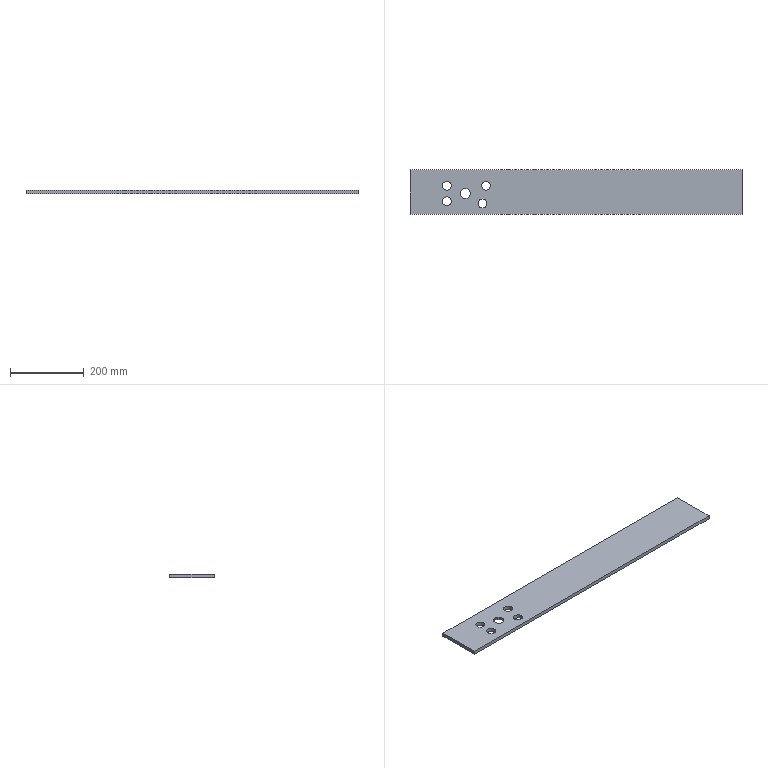Part | STEP file | zhiheceban1 | 1 solid | 13 faces | box 900 x 120 x 10 mm | volume 1052932 mm3 | plane 7 | cylinder 6 | commonest cylinder face diameters 24 x4 28 x1 36 x1
STEP:
#1=CARTESIAN_POINT('',(0.,0.,0.));
#2=DIRECTION('',(0.,0.,1.));
#3=DIRECTION('',(1.,0.,0.));
#4=AXIS2_PLACEMENT_3D('',#1,#2,#3);
#5=CARTESIAN_POINT('',(450.,-60.,-5.));
#6=VERTEX_POINT('',#5);
#7=CARTESIAN_POINT('',(450.,60.,-5.));
#8=VERTEX_POINT('',#7);
#9=CARTESIAN_POINT('',(450.,60.,-5.));
#10=DIRECTION('',(0.,1.,0.));
#11=VECTOR('',#10,1.);
#12=LINE('',#9,#11);
#13=CARTESIAN_POINT('',(450.,60.,5.));
#14=DIRECTION('',(-1.,0.,0.));
#15=DIRECTION('',(0.,0.,1.));
#16=AXIS2_PLACEMENT_3D('',#13,#14,#15);
#17=PLANE('',#16);
#18=CARTESIAN_POINT('',(-10.,0.));
#19=DIRECTION('',(0.,1.));
#20=VECTOR('',#19,1.);
#21=LINE('',#18,#20);
#22=(GEOMETRIC_REPRESENTATION_CONTEXT(2)PARAMETRIC_REPRESENTATION_CONTEXT()REPRESENTATION_CONTEXT('',''));
#23=DEFINITIONAL_REPRESENTATION('',(#21),#22);
#24=PCURVE('',#17,#23);
#25=CARTESIAN_POINT('',(0.,0.,-5.));
#26=DIRECTION('',(0.,0.,1.));
#27=DIRECTION('',(1.,0.,0.));
#28=AXIS2_PLACEMENT_3D('',#25,#26,#27);
#29=PLANE('',#28);
#30=CARTESIAN_POINT('',(450.,60.));
#31=DIRECTION('',(0.,1.));
#32=VECTOR('',#31,1.);
#33=LINE('',#30,#32);
#34=(GEOMETRIC_REPRESENTATION_CONTEXT(2)PARAMETRIC_REPRESENTATION_CONTEXT()REPRESENTATION_CONTEXT('',''));
#35=DEFINITIONAL_REPRESENTATION('',(#33),#34);
#36=PCURVE('',#29,#35);
#37=SURFACE_CURVE('',#12,(#24,#36),.PCURVE_S1.);
#38=EDGE_CURVE('',#6,#8,#37,.T.);
#39=ORIENTED_EDGE('',*,*,#38,.T.);
#40=CARTESIAN_POINT('',(450.,60.,5.));
#41=VERTEX_POINT('',#40);
#42=CARTESIAN_POINT('',(450.,60.,5.));
#43=DIRECTION('',(0.,0.,-1.));
#44=VECTOR('',#43,1.);
#45=LINE('',#42,#44);
#46=CARTESIAN_POINT('',(0.,0.));
#47=DIRECTION('',(-1.,0.));
#48=VECTOR('',#47,1.);
#49=LINE('',#46,#48);
#50=(GEOMETRIC_REPRESENTATION_CONTEXT(2)PARAMETRIC_REPRESENTATION_CONTEXT()REPRESENTATION_CONTEXT('',''));
#51=DEFINITIONAL_REPRESENTATION('',(#49),#50);
#52=PCURVE('',#17,#51);
#53=CARTESIAN_POINT('',(-450.,60.,5.));
#54=DIRECTION('',(0.,-1.,0.));
#55=DIRECTION('',(0.,0.,-1.));
#56=AXIS2_PLACEMENT_3D('',#53,#54,#55);
#57=PLANE('',#56);
#58=CARTESIAN_POINT('',(0.,900.));
#59=DIRECTION('',(1.,0.));
#60=VECTOR('',#59,1.);
#61=LINE('',#58,#60);
#62=(GEOMETRIC_REPRESENTATION_CONTEXT(2)PARAMETRIC_REPRESENTATION_CONTEXT()REPRESENTATION_CONTEXT('',''));
#63=DEFINITIONAL_REPRESENTATION('',(#61),#62);
#64=PCURVE('',#57,#63);
#65=SURFACE_CURVE('',#45,(#52,#64),.PCURVE_S1.);
#66=EDGE_CURVE('',#41,#8,#65,.T.);
#67=ORIENTED_EDGE('',*,*,#66,.F.);
#68=CARTESIAN_POINT('',(450.,-60.,5.));
#69=VERTEX_POINT('',#68);
#70=CARTESIAN_POINT('',(450.,60.,5.));
#71=DIRECTION('',(0.,1.,0.));
#72=VECTOR('',#71,1.);
#73=LINE('',#70,#72);
#74=CARTESIAN_POINT('',(0.,0.));
#75=DIRECTION('',(0.,1.));
#76=VECTOR('',#75,1.);
#77=LINE('',#74,#76);
#78=(GEOMETRIC_REPRESENTATION_CONTEXT(2)PARAMETRIC_REPRESENTATION_CONTEXT()REPRESENTATION_CONTEXT('',''));
#79=DEFINITIONAL_REPRESENTATION('',(#77),#78);
#80=PCURVE('',#17,#79);
#81=CARTESIAN_POINT('',(0.,0.,5.));
#82=DIRECTION('',(0.,0.,1.));
#83=DIRECTION('',(1.,0.,0.));
#84=AXIS2_PLACEMENT_3D('',#81,#82,#83);
#85=PLANE('',#84);
#86=CARTESIAN_POINT('',(450.,60.));
#87=DIRECTION('',(0.,1.));
#88=VECTOR('',#87,1.);
#89=LINE('',#86,#88);
#90=(GEOMETRIC_REPRESENTATION_CONTEXT(2)PARAMETRIC_REPRESENTATION_CONTEXT()REPRESENTATION_CONTEXT('',''));
#91=DEFINITIONAL_REPRESENTATION('',(#89),#90);
#92=PCURVE('',#85,#91);
#93=SURFACE_CURVE('',#73,(#80,#92),.PCURVE_S1.);
#94=EDGE_CURVE('',#69,#41,#93,.T.);
#95=ORIENTED_EDGE('',*,*,#94,.F.);
#96=CARTESIAN_POINT('',(450.,-60.,5.));
#97=DIRECTION('',(0.,0.,-1.));
#98=VECTOR('',#97,1.);
#99=LINE('',#96,#98);
#100=CARTESIAN_POINT('',(0.,-120.));
#101=DIRECTION('',(-1.,0.));
#102=VECTOR('',#101,1.);
#103=LINE('',#100,#102);
#104=(GEOMETRIC_REPRESENTATION_CONTEXT(2)PARAMETRIC_REPRESENTATION_CONTEXT()REPRESENTATION_CONTEXT('',''));
#105=DEFINITIONAL_REPRESENTATION('',(#103),#104);
#106=PCURVE('',#17,#105);
#107=CARTESIAN_POINT('',(-450.,-60.,5.));
#108=DIRECTION('',(0.,1.,0.));
#109=DIRECTION('',(0.,0.,1.));
#110=AXIS2_PLACEMENT_3D('',#107,#108,#109);
#111=PLANE('',#110);
#112=CARTESIAN_POINT('',(0.,900.));
#113=DIRECTION('',(-1.,0.));
#114=VECTOR('',#113,1.);
#115=LINE('',#112,#114);
#116=(GEOMETRIC_REPRESENTATION_CONTEXT(2)PARAMETRIC_REPRESENTATION_CONTEXT()REPRESENTATION_CONTEXT('',''));
#117=DEFINITIONAL_REPRESENTATION('',(#115),#116);
#118=PCURVE('',#111,#117);
#119=SURFACE_CURVE('',#99,(#106,#118),.PCURVE_S1.);
#120=EDGE_CURVE('',#69,#6,#119,.T.);
#121=ORIENTED_EDGE('',*,*,#120,.T.);
#122=EDGE_LOOP('',(#39,#67,#95,#121));
#123=FACE_BOUND('',#122,.T.);
#124=ADVANCED_FACE('',(#123),#17,.F.);
#125=CARTESIAN_POINT('',(-450.,60.,-5.));
#126=VERTEX_POINT('',#125);
#127=CARTESIAN_POINT('',(-450.,60.,-5.));
#128=DIRECTION('',(-1.,0.,0.));
#129=VECTOR('',#128,1.);
#130=LINE('',#127,#129);
#131=CARTESIAN_POINT('',(10.,0.));
#132=DIRECTION('',(0.,-1.));
#133=VECTOR('',#132,1.);
#134=LINE('',#131,#133);
#135=(GEOMETRIC_REPRESENTATION_CONTEXT(2)PARAMETRIC_REPRESENTATION_CONTEXT()REPRESENTATION_CONTEXT('',''));
#136=DEFINITIONAL_REPRESENTATION('',(#134),#135);
#137=PCURVE('',#57,#136);
#138=CARTESIAN_POINT('',(-450.,60.));
#139=DIRECTION('',(-1.,0.));
#140=VECTOR('',#139,1.);
#141=LINE('',#138,#140);
#142=(GEOMETRIC_REPRESENTATION_CONTEXT(2)PARAMETRIC_REPRESENTATION_CONTEXT()REPRESENTATION_CONTEXT('',''));
#143=DEFINITIONAL_REPRESENTATION('',(#141),#142);
#144=PCURVE('',#29,#143);
#145=SURFACE_CURVE('',#130,(#137,#144),.PCURVE_S1.);
#146=EDGE_CURVE('',#8,#126,#145,.T.);
#147=ORIENTED_EDGE('',*,*,#146,.T.);
#148=CARTESIAN_POINT('',(-450.,60.,5.));
#149=VERTEX_POINT('',#148);
#150=CARTESIAN_POINT('',(-450.,60.,5.));
#151=DIRECTION('',(0.,0.,-1.));
#152=VECTOR('',#151,1.);
#153=LINE('',#150,#152);
#154=CARTESIAN_POINT('',(0.,0.));
#155=DIRECTION('',(1.,0.));
#156=VECTOR('',#155,1.);
#157=LINE('',#154,#156);
#158=(GEOMETRIC_REPRESENTATION_CONTEXT(2)PARAMETRIC_REPRESENTATION_CONTEXT()REPRESENTATION_CONTEXT('',''));
#159=DEFINITIONAL_REPRESENTATION('',(#157),#158);
#160=PCURVE('',#57,#159);
#161=CARTESIAN_POINT('',(-450.,60.,5.));
#162=DIRECTION('',(1.,0.,0.));
#163=DIRECTION('',(0.,0.,-1.));
#164=AXIS2_PLACEMENT_3D('',#161,#162,#163);
#165=PLANE('',#164);
#166=CARTESIAN_POINT('',(0.,0.));
#167=DIRECTION('',(1.,0.));
#168=VECTOR('',#167,1.);
#169=LINE('',#166,#168);
#170=(GEOMETRIC_REPRESENTATION_CONTEXT(2)PARAMETRIC_REPRESENTATION_CONTEXT()REPRESENTATION_CONTEXT('',''));
#171=DEFINITIONAL_REPRESENTATION('',(#169),#170);
#172=PCURVE('',#165,#171);
#173=SURFACE_CURVE('',#153,(#160,#172),.PCURVE_S1.);
#174=EDGE_CURVE('',#149,#126,#173,.T.);
#175=ORIENTED_EDGE('',*,*,#174,.F.);
#176=CARTESIAN_POINT('',(-450.,60.,5.));
#177=DIRECTION('',(-1.,0.,0.));
#178=VECTOR('',#177,1.);
#179=LINE('',#176,#178);
#180=CARTESIAN_POINT('',(0.,0.));
#181=DIRECTION('',(0.,-1.));
#182=VECTOR('',#181,1.);
#183=LINE('',#180,#182);
#184=(GEOMETRIC_REPRESENTATION_CONTEXT(2)PARAMETRIC_REPRESENTATION_CONTEXT()REPRESENTATION_CONTEXT('',''));
#185=DEFINITIONAL_REPRESENTATION('',(#183),#184);
#186=PCURVE('',#57,#185);
#187=CARTESIAN_POINT('',(-450.,60.));
#188=DIRECTION('',(-1.,0.));
#189=VECTOR('',#188,1.);
#190=LINE('',#187,#189);
#191=(GEOMETRIC_REPRESENTATION_CONTEXT(2)PARAMETRIC_REPRESENTATION_CONTEXT()REPRESENTATION_CONTEXT('',''));
#192=DEFINITIONAL_REPRESENTATION('',(#190),#191);
#193=PCURVE('',#85,#192);
#194=SURFACE_CURVE('',#179,(#186,#193),.PCURVE_S1.);
#195=EDGE_CURVE('',#41,#149,#194,.T.);
#196=ORIENTED_EDGE('',*,*,#195,.F.);
#197=ORIENTED_EDGE('',*,*,#66,.T.);
#198=EDGE_LOOP('',(#147,#175,#196,#197));
#199=FACE_BOUND('',#198,.T.);
#200=ADVANCED_FACE('',(#199),#57,.F.);
#201=CARTESIAN_POINT('',(-450.,-60.,-5.));
#202=VERTEX_POINT('',#201);
#203=CARTESIAN_POINT('',(-450.,60.,-5.));
#204=DIRECTION('',(0.,-1.,0.));
#205=VECTOR('',#204,1.);
#206=LINE('',#203,#205);
#207=CARTESIAN_POINT('',(10.,0.));
#208=DIRECTION('',(0.,-1.));
#209=VECTOR('',#208,1.);
#210=LINE('',#207,#209);
#211=(GEOMETRIC_REPRESENTATION_CONTEXT(2)PARAMETRIC_REPRESENTATION_CONTEXT()REPRESENTATION_CONTEXT('',''));
#212=DEFINITIONAL_REPRESENTATION('',(#210),#211);
#213=PCURVE('',#165,#212);
#214=CARTESIAN_POINT('',(-450.,60.));
#215=DIRECTION('',(0.,-1.));
#216=VECTOR('',#215,1.);
#217=LINE('',#214,#216);
#218=(GEOMETRIC_REPRESENTATION_CONTEXT(2)PARAMETRIC_REPRESENTATION_CONTEXT()REPRESENTATION_CONTEXT('',''));
#219=DEFINITIONAL_REPRESENTATION('',(#217),#218);
#220=PCURVE('',#29,#219);
#221=SURFACE_CURVE('',#206,(#213,#220),.PCURVE_S1.);
#222=EDGE_CURVE('',#126,#202,#221,.T.);
#223=ORIENTED_EDGE('',*,*,#222,.T.);
#224=CARTESIAN_POINT('',(-450.,-60.,5.));
#225=VERTEX_POINT('',#224);
#226=CARTESIAN_POINT('',(-450.,-60.,5.));
#227=DIRECTION('',(0.,0.,-1.));
#228=VECTOR('',#227,1.);
#229=LINE('',#226,#228);
#230=CARTESIAN_POINT('',(0.,-120.));
#231=DIRECTION('',(1.,0.));
#232=VECTOR('',#231,1.);
#233=LINE('',#230,#232);
#234=(GEOMETRIC_REPRESENTATION_CONTEXT(2)PARAMETRIC_REPRESENTATION_CONTEXT()REPRESENTATION_CONTEXT('',''));
#235=DEFINITIONAL_REPRESENTATION('',(#233),#234);
#236=PCURVE('',#165,#235);
#237=CARTESIAN_POINT('',(0.,0.));
#238=DIRECTION('',(-1.,0.));
#239=VECTOR('',#238,1.);
#240=LINE('',#237,#239);
#241=(GEOMETRIC_REPRESENTATION_CONTEXT(2)PARAMETRIC_REPRESENTATION_CONTEXT()REPRESENTATION_CONTEXT('',''));
#242=DEFINITIONAL_REPRESENTATION('',(#240),#241);
#243=PCURVE('',#111,#242);
#244=SURFACE_CURVE('',#229,(#236,#243),.PCURVE_S1.);
#245=EDGE_CURVE('',#225,#202,#244,.T.);
#246=ORIENTED_EDGE('',*,*,#245,.F.);
#247=CARTESIAN_POINT('',(-450.,60.,5.));
#248=DIRECTION('',(0.,-1.,0.));
#249=VECTOR('',#248,1.);
#250=LINE('',#247,#249);
#251=CARTESIAN_POINT('',(0.,0.));
#252=DIRECTION('',(0.,-1.));
#253=VECTOR('',#252,1.);
#254=LINE('',#251,#253);
#255=(GEOMETRIC_REPRESENTATION_CONTEXT(2)PARAMETRIC_REPRESENTATION_CONTEXT()REPRESENTATION_CONTEXT('',''));
#256=DEFINITIONAL_REPRESENTATION('',(#254),#255);
#257=PCURVE('',#165,#256);
#258=CARTESIAN_POINT('',(-450.,60.));
#259=DIRECTION('',(0.,-1.));
#260=VECTOR('',#259,1.);
#261=LINE('',#258,#260);
#262=(GEOMETRIC_REPRESENTATION_CONTEXT(2)PARAMETRIC_REPRESENTATION_CONTEXT()REPRESENTATION_CONTEXT('',''));
#263=DEFINITIONAL_REPRESENTATION('',(#261),#262);
#264=PCURVE('',#85,#263);
#265=SURFACE_CURVE('',#250,(#257,#264),.PCURVE_S1.);
#266=EDGE_CURVE('',#149,#225,#265,.T.);
#267=ORIENTED_EDGE('',*,*,#266,.F.);
#268=ORIENTED_EDGE('',*,*,#174,.T.);
#269=EDGE_LOOP('',(#223,#246,#267,#268));
#270=FACE_BOUND('',#269,.T.);
#271=ADVANCED_FACE('',(#270),#165,.F.);
#272=CARTESIAN_POINT('',(-450.,-60.,-5.));
#273=DIRECTION('',(1.,0.,0.));
#274=VECTOR('',#273,1.);
#275=LINE('',#272,#274);
#276=CARTESIAN_POINT('',(-10.,0.));
#277=DIRECTION('',(0.,1.));
#278=VECTOR('',#277,1.);
#279=LINE('',#276,#278);
#280=(GEOMETRIC_REPRESENTATION_CONTEXT(2)PARAMETRIC_REPRESENTATION_CONTEXT()REPRESENTATION_CONTEXT('',''));
#281=DEFINITIONAL_REPRESENTATION('',(#279),#280);
#282=PCURVE('',#111,#281);
#283=CARTESIAN_POINT('',(-450.,-60.));
#284=DIRECTION('',(1.,0.));
#285=VECTOR('',#284,1.);
#286=LINE('',#283,#285);
#287=(GEOMETRIC_REPRESENTATION_CONTEXT(2)PARAMETRIC_REPRESENTATION_CONTEXT()REPRESENTATION_CONTEXT('',''));
#288=DEFINITIONAL_REPRESENTATION('',(#286),#287);
#289=PCURVE('',#29,#288);
#290=SURFACE_CURVE('',#275,(#282,#289),.PCURVE_S1.);
#291=EDGE_CURVE('',#202,#6,#290,.T.);
#292=ORIENTED_EDGE('',*,*,#291,.T.);
#293=ORIENTED_EDGE('',*,*,#120,.F.);
#294=CARTESIAN_POINT('',(-450.,-60.,5.));
#295=DIRECTION('',(1.,0.,0.));
#296=VECTOR('',#295,1.);
#297=LINE('',#294,#296);
#298=CARTESIAN_POINT('',(0.,0.));
#299=DIRECTION('',(0.,1.));
#300=VECTOR('',#299,1.);
#301=LINE('',#298,#300);
#302=(GEOMETRIC_REPRESENTATION_CONTEXT(2)PARAMETRIC_REPRESENTATION_CONTEXT()REPRESENTATION_CONTEXT('',''));
#303=DEFINITIONAL_REPRESENTATION('',(#301),#302);
#304=PCURVE('',#111,#303);
#305=CARTESIAN_POINT('',(-450.,-60.));
#306=DIRECTION('',(1.,0.));
#307=VECTOR('',#306,1.);
#308=LINE('',#305,#307);
#309=(GEOMETRIC_REPRESENTATION_CONTEXT(2)PARAMETRIC_REPRESENTATION_CONTEXT()REPRESENTATION_CONTEXT('',''));
#310=DEFINITIONAL_REPRESENTATION('',(#308),#309);
#311=PCURVE('',#85,#310);
#312=SURFACE_CURVE('',#297,(#304,#311),.PCURVE_S1.);
#313=EDGE_CURVE('',#225,#69,#312,.T.);
#314=ORIENTED_EDGE('',*,*,#313,.F.);
#315=ORIENTED_EDGE('',*,*,#245,.T.);
#316=EDGE_LOOP('',(#292,#293,#314,#315));
#317=FACE_BOUND('',#316,.T.);
#318=ADVANCED_FACE('',(#317),#111,.F.);
#319=CARTESIAN_POINT('',(-265.485,-31.,5.));
#320=VERTEX_POINT('',#319);
#321=CARTESIAN_POINT('',(-253.485,-31.,5.));
#322=DIRECTION('',(0.,0.,-1.));
#323=DIRECTION('',(-1.,0.,0.));
#324=AXIS2_PLACEMENT_3D('',#321,#322,#323);
#325=CIRCLE('',#324,12.);
#326=CARTESIAN_POINT('',(-265.485,-31.));
#327=CARTESIAN_POINT('',(-265.485,-10.215));
#328=CARTESIAN_POINT('',(-247.485,-20.608));
#329=CARTESIAN_POINT('',(-229.485,-31.));
#330=CARTESIAN_POINT('',(-247.485,-41.392));
#331=CARTESIAN_POINT('',(-265.485,-51.785));
#332=CARTESIAN_POINT('',(-265.485,-31.));
#333=(BOUNDED_CURVE()B_SPLINE_CURVE(2,(#326,#327,#328,#329,#330,#331,#332),.UNSPECIFIED.,.T.,.F.)B_SPLINE_CURVE_WITH_KNOTS((1,2,2,2,2,1),(-2.094,0.,2.094,4.189,6.283,8.378),.UNSPECIFIED.)CURVE()GEOMETRIC_REPRESENTATION_ITEM()RATIONAL_B_SPLINE_CURVE((1.,0.5,1.,0.5,1.,0.5,1.))REPRESENTATION_ITEM(''));
#334=(GEOMETRIC_REPRESENTATION_CONTEXT(2)PARAMETRIC_REPRESENTATION_CONTEXT()REPRESENTATION_CONTEXT('',''));
#335=DEFINITIONAL_REPRESENTATION('',(#333),#334);
#336=PCURVE('',#85,#335);
#337=CARTESIAN_POINT('',(-253.485,-31.,5.));
#338=DIRECTION('',(0.,0.,-1.));
#339=DIRECTION('',(-1.,0.,0.));
#340=AXIS2_PLACEMENT_3D('',#337,#338,#339);
#341=CYLINDRICAL_SURFACE('',#340,12.);
#342=CARTESIAN_POINT('',(0.,0.));
#343=DIRECTION('',(1.,0.));
#344=VECTOR('',#343,1.);
#345=LINE('',#342,#344);
#346=(GEOMETRIC_REPRESENTATION_CONTEXT(2)PARAMETRIC_REPRESENTATION_CONTEXT()REPRESENTATION_CONTEXT('',''));
#347=DEFINITIONAL_REPRESENTATION('',(#345),#346);
#348=PCURVE('',#341,#347);
#349=SURFACE_CURVE('',#325,(#336,#348),.PCURVE_S1.);
#350=EDGE_CURVE('',#320,#320,#349,.T.);
#351=ORIENTED_EDGE('',*,*,#350,.T.);
#352=EDGE_LOOP('',(#351));
#353=FACE_BOUND('',#352,.T.);
#354=CARTESIAN_POINT('',(-314.251,-4.,5.));
#355=VERTEX_POINT('',#354);
#356=CARTESIAN_POINT('',(-300.251,-4.,5.));
#357=DIRECTION('',(0.,0.,-1.));
#358=DIRECTION('',(-1.,0.,0.));
#359=AXIS2_PLACEMENT_3D('',#356,#357,#358);
#360=CIRCLE('',#359,14.);
#361=CARTESIAN_POINT('',(-314.251,-4.));
#362=CARTESIAN_POINT('',(-314.251,20.249));
#363=CARTESIAN_POINT('',(-293.251,8.124));
#364=CARTESIAN_POINT('',(-272.251,-4.));
#365=CARTESIAN_POINT('',(-293.251,-16.124));
#366=CARTESIAN_POINT('',(-314.251,-28.249));
#367=CARTESIAN_POINT('',(-314.251,-4.));
#368=(BOUNDED_CURVE()B_SPLINE_CURVE(2,(#361,#362,#363,#364,#365,#366,#367),.UNSPECIFIED.,.T.,.F.)B_SPLINE_CURVE_WITH_KNOTS((1,2,2,2,2,1),(-2.094,0.,2.094,4.189,6.283,8.378),.UNSPECIFIED.)CURVE()GEOMETRIC_REPRESENTATION_ITEM()RATIONAL_B_SPLINE_CURVE((1.,0.5,1.,0.5,1.,0.5,1.))REPRESENTATION_ITEM(''));
#369=(GEOMETRIC_REPRESENTATION_CONTEXT(2)PARAMETRIC_REPRESENTATION_CONTEXT()REPRESENTATION_CONTEXT('',''));
#370=DEFINITIONAL_REPRESENTATION('',(#368),#369);
#371=PCURVE('',#85,#370);
#372=CARTESIAN_POINT('',(-300.251,-4.,5.));
#373=DIRECTION('',(0.,0.,-1.));
#374=DIRECTION('',(-1.,0.,0.));
#375=AXIS2_PLACEMENT_3D('',#372,#373,#374);
#376=CYLINDRICAL_SURFACE('',#375,14.);
#377=CARTESIAN_POINT('',(0.,0.));
#378=DIRECTION('',(1.,0.));
#379=VECTOR('',#378,1.);
#380=LINE('',#377,#379);
#381=(GEOMETRIC_REPRESENTATION_CONTEXT(2)PARAMETRIC_REPRESENTATION_CONTEXT()REPRESENTATION_CONTEXT('',''));
#382=DEFINITIONAL_REPRESENTATION('',(#380),#381);
#383=PCURVE('',#376,#382);
#384=SURFACE_CURVE('',#360,(#371,#383),.PCURVE_S1.);
#385=EDGE_CURVE('',#355,#355,#384,.T.);
#386=ORIENTED_EDGE('',*,*,#385,.T.);
#387=EDGE_LOOP('',(#386));
#388=FACE_BOUND('',#387,.T.);
#389=CARTESIAN_POINT('',(-362.,17.,5.));
#390=VERTEX_POINT('',#389);
#391=CARTESIAN_POINT('',(-350.,17.,5.));
#392=DIRECTION('',(0.,0.,-1.));
#393=DIRECTION('',(-1.,0.,0.));
#394=AXIS2_PLACEMENT_3D('',#391,#392,#393);
#395=CIRCLE('',#394,12.);
#396=CARTESIAN_POINT('',(-362.,17.));
#397=CARTESIAN_POINT('',(-362.,37.785));
#398=CARTESIAN_POINT('',(-344.,27.392));
#399=CARTESIAN_POINT('',(-326.,17.));
#400=CARTESIAN_POINT('',(-344.,6.608));
#401=CARTESIAN_POINT('',(-362.,-3.785));
#402=CARTESIAN_POINT('',(-362.,17.));
#403=(BOUNDED_CURVE()B_SPLINE_CURVE(2,(#396,#397,#398,#399,#400,#401,#402),.UNSPECIFIED.,.T.,.F.)B_SPLINE_CURVE_WITH_KNOTS((1,2,2,2,2,1),(-2.094,0.,2.094,4.189,6.283,8.378),.UNSPECIFIED.)CURVE()GEOMETRIC_REPRESENTATION_ITEM()RATIONAL_B_SPLINE_CURVE((1.,0.5,1.,0.5,1.,0.5,1.))REPRESENTATION_ITEM(''));
#404=(GEOMETRIC_REPRESENTATION_CONTEXT(2)PARAMETRIC_REPRESENTATION_CONTEXT()REPRESENTATION_CONTEXT('',''));
#405=DEFINITIONAL_REPRESENTATION('',(#403),#404);
#406=PCURVE('',#85,#405);
#407=CARTESIAN_POINT('',(-350.,17.,5.));
#408=DIRECTION('',(0.,0.,-1.));
#409=DIRECTION('',(-1.,0.,0.));
#410=AXIS2_PLACEMENT_3D('',#407,#408,#409);
#411=CYLINDRICAL_SURFACE('',#410,12.);
#412=CARTESIAN_POINT('',(0.,0.));
#413=DIRECTION('',(1.,0.));
#414=VECTOR('',#413,1.);
#415=LINE('',#412,#414);
#416=(GEOMETRIC_REPRESENTATION_CONTEXT(2)PARAMETRIC_REPRESENTATION_CONTEXT()REPRESENTATION_CONTEXT('',''));
#417=DEFINITIONAL_REPRESENTATION('',(#415),#416);
#418=PCURVE('',#411,#417);
#419=SURFACE_CURVE('',#395,(#406,#418),.PCURVE_S1.);
#420=EDGE_CURVE('',#390,#390,#419,.T.);
#421=ORIENTED_EDGE('',*,*,#420,.T.);
#422=EDGE_LOOP('',(#421));
#423=FACE_BOUND('',#422,.T.);
#424=CARTESIAN_POINT('',(-362.,-25.,5.));
#425=VERTEX_POINT('',#424);
#426=CARTESIAN_POINT('',(-350.,-25.,5.));
#427=DIRECTION('',(0.,0.,-1.));
#428=DIRECTION('',(-1.,0.,0.));
#429=AXIS2_PLACEMENT_3D('',#426,#427,#428);
#430=CIRCLE('',#429,12.);
#431=CARTESIAN_POINT('',(-362.,-25.));
#432=CARTESIAN_POINT('',(-362.,-4.215));
#433=CARTESIAN_POINT('',(-344.,-14.608));
#434=CARTESIAN_POINT('',(-326.,-25.));
#435=CARTESIAN_POINT('',(-344.,-35.392));
#436=CARTESIAN_POINT('',(-362.,-45.785));
#437=CARTESIAN_POINT('',(-362.,-25.));
#438=(BOUNDED_CURVE()B_SPLINE_CURVE(2,(#431,#432,#433,#434,#435,#436,#437),.UNSPECIFIED.,.T.,.F.)B_SPLINE_CURVE_WITH_KNOTS((1,2,2,2,2,1),(-2.094,0.,2.094,4.189,6.283,8.378),.UNSPECIFIED.)CURVE()GEOMETRIC_REPRESENTATION_ITEM()RATIONAL_B_SPLINE_CURVE((1.,0.5,1.,0.5,1.,0.5,1.))REPRESENTATION_ITEM(''));
#439=(GEOMETRIC_REPRESENTATION_CONTEXT(2)PARAMETRIC_REPRESENTATION_CONTEXT()REPRESENTATION_CONTEXT('',''));
#440=DEFINITIONAL_REPRESENTATION('',(#438),#439);
#441=PCURVE('',#85,#440);
#442=CARTESIAN_POINT('',(-350.,-25.,5.));
#443=DIRECTION('',(0.,0.,-1.));
#444=DIRECTION('',(-1.,0.,0.));
#445=AXIS2_PLACEMENT_3D('',#442,#443,#444);
#446=CYLINDRICAL_SURFACE('',#445,12.);
#447=CARTESIAN_POINT('',(0.,0.));
#448=DIRECTION('',(1.,0.));
#449=VECTOR('',#448,1.);
#450=LINE('',#447,#449);
#451=(GEOMETRIC_REPRESENTATION_CONTEXT(2)PARAMETRIC_REPRESENTATION_CONTEXT()REPRESENTATION_CONTEXT('',''));
#452=DEFINITIONAL_REPRESENTATION('',(#450),#451);
#453=PCURVE('',#446,#452);
#454=SURFACE_CURVE('',#430,(#441,#453),.PCURVE_S1.);
#455=EDGE_CURVE('',#425,#425,#454,.T.);
#456=ORIENTED_EDGE('',*,*,#455,.T.);
#457=EDGE_LOOP('',(#456));
#458=FACE_BOUND('',#457,.T.);
#459=CARTESIAN_POINT('',(-256.046,17.,5.));
#460=VERTEX_POINT('',#459);
#461=CARTESIAN_POINT('',(-244.046,17.,5.));
#462=DIRECTION('',(0.,0.,-1.));
#463=DIRECTION('',(-1.,0.,0.));
#464=AXIS2_PLACEMENT_3D('',#461,#462,#463);
#465=CIRCLE('',#464,12.);
#466=CARTESIAN_POINT('',(-256.046,17.));
#467=CARTESIAN_POINT('',(-256.046,37.785));
#468=CARTESIAN_POINT('',(-238.046,27.392));
#469=CARTESIAN_POINT('',(-220.046,17.));
#470=CARTESIAN_POINT('',(-238.046,6.608));
#471=CARTESIAN_POINT('',(-256.046,-3.785));
#472=CARTESIAN_POINT('',(-256.046,17.));
#473=(BOUNDED_CURVE()B_SPLINE_CURVE(2,(#466,#467,#468,#469,#470,#471,#472),.UNSPECIFIED.,.T.,.F.)B_SPLINE_CURVE_WITH_KNOTS((1,2,2,2,2,1),(-2.094,0.,2.094,4.189,6.283,8.378),.UNSPECIFIED.)CURVE()GEOMETRIC_REPRESENTATION_ITEM()RATIONAL_B_SPLINE_CURVE((1.,0.5,1.,0.5,1.,0.5,1.))REPRESENTATION_ITEM(''));
#474=(GEOMETRIC_REPRESENTATION_CONTEXT(2)PARAMETRIC_REPRESENTATION_CONTEXT()REPRESENTATION_CONTEXT('',''));
#475=DEFINITIONAL_REPRESENTATION('',(#473),#474);
#476=PCURVE('',#85,#475);
#477=CARTESIAN_POINT('',(-244.046,17.,5.));
#478=DIRECTION('',(0.,0.,-1.));
#479=DIRECTION('',(-1.,0.,0.));
#480=AXIS2_PLACEMENT_3D('',#477,#478,#479);
#481=CYLINDRICAL_SURFACE('',#480,12.);
#482=CARTESIAN_POINT('',(0.,0.));
#483=DIRECTION('',(1.,0.));
#484=VECTOR('',#483,1.);
#485=LINE('',#482,#484);
#486=(GEOMETRIC_REPRESENTATION_CONTEXT(2)PARAMETRIC_REPRESENTATION_CONTEXT()REPRESENTATION_CONTEXT('',''));
#487=DEFINITIONAL_REPRESENTATION('',(#485),#486);
#488=PCURVE('',#481,#487);
#489=SURFACE_CURVE('',#465,(#476,#488),.PCURVE_S1.);
#490=EDGE_CURVE('',#460,#460,#489,.T.);
#491=ORIENTED_EDGE('',*,*,#490,.T.);
#492=EDGE_LOOP('',(#491));
#493=FACE_BOUND('',#492,.T.);
#494=ORIENTED_EDGE('',*,*,#94,.T.);
#495=ORIENTED_EDGE('',*,*,#195,.T.);
#496=ORIENTED_EDGE('',*,*,#266,.T.);
#497=ORIENTED_EDGE('',*,*,#313,.T.);
#498=EDGE_LOOP('',(#494,#495,#496,#497));
#499=FACE_BOUND('',#498,.T.);
#500=ADVANCED_FACE('',(#353,#388,#423,#458,#493,#499),#85,.T.);
#501=CARTESIAN_POINT('',(-265.485,-31.,-5.));
#502=VERTEX_POINT('',#501);
#503=CARTESIAN_POINT('',(-253.485,-31.,-5.));
#504=DIRECTION('',(0.,0.,-1.));
#505=DIRECTION('',(-1.,0.,0.));
#506=AXIS2_PLACEMENT_3D('',#503,#504,#505);
#507=CIRCLE('',#506,12.);
#508=CARTESIAN_POINT('',(-265.485,-31.));
#509=CARTESIAN_POINT('',(-265.485,-10.215));
#510=CARTESIAN_POINT('',(-247.485,-20.608));
#511=CARTESIAN_POINT('',(-229.485,-31.));
#512=CARTESIAN_POINT('',(-247.485,-41.392));
#513=CARTESIAN_POINT('',(-265.485,-51.785));
#514=CARTESIAN_POINT('',(-265.485,-31.));
#515=(BOUNDED_CURVE()B_SPLINE_CURVE(2,(#508,#509,#510,#511,#512,#513,#514),.UNSPECIFIED.,.T.,.F.)B_SPLINE_CURVE_WITH_KNOTS((1,2,2,2,2,1),(-2.094,0.,2.094,4.189,6.283,8.378),.UNSPECIFIED.)CURVE()GEOMETRIC_REPRESENTATION_ITEM()RATIONAL_B_SPLINE_CURVE((1.,0.5,1.,0.5,1.,0.5,1.))REPRESENTATION_ITEM(''));
#516=(GEOMETRIC_REPRESENTATION_CONTEXT(2)PARAMETRIC_REPRESENTATION_CONTEXT()REPRESENTATION_CONTEXT('',''));
#517=DEFINITIONAL_REPRESENTATION('',(#515),#516);
#518=PCURVE('',#29,#517);
#519=CARTESIAN_POINT('',(0.,10.));
#520=DIRECTION('',(1.,0.));
#521=VECTOR('',#520,1.);
#522=LINE('',#519,#521);
#523=(GEOMETRIC_REPRESENTATION_CONTEXT(2)PARAMETRIC_REPRESENTATION_CONTEXT()REPRESENTATION_CONTEXT('',''));
#524=DEFINITIONAL_REPRESENTATION('',(#522),#523);
#525=PCURVE('',#341,#524);
#526=SURFACE_CURVE('',#507,(#518,#525),.PCURVE_S1.);
#527=EDGE_CURVE('',#502,#502,#526,.T.);
#528=ORIENTED_EDGE('',*,*,#527,.F.);
#529=EDGE_LOOP('',(#528));
#530=FACE_BOUND('',#529,.T.);
#531=CARTESIAN_POINT('',(-318.251,-4.,-5.));
#532=VERTEX_POINT('',#531);
#533=CARTESIAN_POINT('',(-300.251,-4.,-5.));
#534=DIRECTION('',(0.,0.,-1.));
#535=DIRECTION('',(-1.,0.,0.));
#536=AXIS2_PLACEMENT_3D('',#533,#534,#535);
#537=CIRCLE('',#536,18.);
#538=CARTESIAN_POINT('',(-318.251,-4.));
#539=CARTESIAN_POINT('',(-318.251,27.177));
#540=CARTESIAN_POINT('',(-291.251,11.588));
#541=CARTESIAN_POINT('',(-264.251,-4.));
#542=CARTESIAN_POINT('',(-291.251,-19.588));
#543=CARTESIAN_POINT('',(-318.251,-35.177));
#544=CARTESIAN_POINT('',(-318.251,-4.));
#545=(BOUNDED_CURVE()B_SPLINE_CURVE(2,(#538,#539,#540,#541,#542,#543,#544),.UNSPECIFIED.,.T.,.F.)B_SPLINE_CURVE_WITH_KNOTS((1,2,2,2,2,1),(-2.094,0.,2.094,4.189,6.283,8.378),.UNSPECIFIED.)CURVE()GEOMETRIC_REPRESENTATION_ITEM()RATIONAL_B_SPLINE_CURVE((1.,0.5,1.,0.5,1.,0.5,1.))REPRESENTATION_ITEM(''));
#546=(GEOMETRIC_REPRESENTATION_CONTEXT(2)PARAMETRIC_REPRESENTATION_CONTEXT()REPRESENTATION_CONTEXT('',''));
#547=DEFINITIONAL_REPRESENTATION('',(#545),#546);
#548=PCURVE('',#29,#547);
#549=CARTESIAN_POINT('',(-300.251,-4.,2.));
#550=DIRECTION('',(0.,0.,-1.));
#551=DIRECTION('',(-1.,0.,0.));
#552=AXIS2_PLACEMENT_3D('',#549,#550,#551);
#553=CYLINDRICAL_SURFACE('',#552,18.);
#554=CARTESIAN_POINT('',(0.,7.));
#555=DIRECTION('',(1.,0.));
#556=VECTOR('',#555,1.);
#557=LINE('',#554,#556);
#558=(GEOMETRIC_REPRESENTATION_CONTEXT(2)PARAMETRIC_REPRESENTATION_CONTEXT()REPRESENTATION_CONTEXT('',''));
#559=DEFINITIONAL_REPRESENTATION('',(#557),#558);
#560=PCURVE('',#553,#559);
#561=SURFACE_CURVE('',#537,(#548,#560),.PCURVE_S1.);
#562=EDGE_CURVE('',#532,#532,#561,.T.);
#563=ORIENTED_EDGE('',*,*,#562,.F.);
#564=EDGE_LOOP('',(#563));
#565=FACE_BOUND('',#564,.T.);
#566=CARTESIAN_POINT('',(-362.,17.,-5.));
#567=VERTEX_POINT('',#566);
#568=CARTESIAN_POINT('',(-350.,17.,-5.));
#569=DIRECTION('',(0.,0.,-1.));
#570=DIRECTION('',(-1.,0.,0.));
#571=AXIS2_PLACEMENT_3D('',#568,#569,#570);
#572=CIRCLE('',#571,12.);
#573=CARTESIAN_POINT('',(-362.,17.));
#574=CARTESIAN_POINT('',(-362.,37.785));
#575=CARTESIAN_POINT('',(-344.,27.392));
#576=CARTESIAN_POINT('',(-326.,17.));
#577=CARTESIAN_POINT('',(-344.,6.608));
#578=CARTESIAN_POINT('',(-362.,-3.785));
#579=CARTESIAN_POINT('',(-362.,17.));
#580=(BOUNDED_CURVE()B_SPLINE_CURVE(2,(#573,#574,#575,#576,#577,#578,#579),.UNSPECIFIED.,.T.,.F.)B_SPLINE_CURVE_WITH_KNOTS((1,2,2,2,2,1),(-2.094,0.,2.094,4.189,6.283,8.378),.UNSPECIFIED.)CURVE()GEOMETRIC_REPRESENTATION_ITEM()RATIONAL_B_SPLINE_CURVE((1.,0.5,1.,0.5,1.,0.5,1.))REPRESENTATION_ITEM(''));
#581=(GEOMETRIC_REPRESENTATION_CONTEXT(2)PARAMETRIC_REPRESENTATION_CONTEXT()REPRESENTATION_CONTEXT('',''));
#582=DEFINITIONAL_REPRESENTATION('',(#580),#581);
#583=PCURVE('',#29,#582);
#584=CARTESIAN_POINT('',(0.,10.));
#585=DIRECTION('',(1.,0.));
#586=VECTOR('',#585,1.);
#587=LINE('',#584,#586);
#588=(GEOMETRIC_REPRESENTATION_CONTEXT(2)PARAMETRIC_REPRESENTATION_CONTEXT()REPRESENTATION_CONTEXT('',''));
#589=DEFINITIONAL_REPRESENTATION('',(#587),#588);
#590=PCURVE('',#411,#589);
#591=SURFACE_CURVE('',#572,(#583,#590),.PCURVE_S1.);
#592=EDGE_CURVE('',#567,#567,#591,.T.);
#593=ORIENTED_EDGE('',*,*,#592,.F.);
#594=EDGE_LOOP('',(#593));
#595=FACE_BOUND('',#594,.T.);
#596=CARTESIAN_POINT('',(-362.,-25.,-5.));
#597=VERTEX_POINT('',#596);
#598=CARTESIAN_POINT('',(-350.,-25.,-5.));
#599=DIRECTION('',(0.,0.,-1.));
#600=DIRECTION('',(-1.,0.,0.));
#601=AXIS2_PLACEMENT_3D('',#598,#599,#600);
#602=CIRCLE('',#601,12.);
#603=CARTESIAN_POINT('',(-362.,-25.));
#604=CARTESIAN_POINT('',(-362.,-4.215));
#605=CARTESIAN_POINT('',(-344.,-14.608));
#606=CARTESIAN_POINT('',(-326.,-25.));
#607=CARTESIAN_POINT('',(-344.,-35.392));
#608=CARTESIAN_POINT('',(-362.,-45.785));
#609=CARTESIAN_POINT('',(-362.,-25.));
#610=(BOUNDED_CURVE()B_SPLINE_CURVE(2,(#603,#604,#605,#606,#607,#608,#609),.UNSPECIFIED.,.T.,.F.)B_SPLINE_CURVE_WITH_KNOTS((1,2,2,2,2,1),(-2.094,0.,2.094,4.189,6.283,8.378),.UNSPECIFIED.)CURVE()GEOMETRIC_REPRESENTATION_ITEM()RATIONAL_B_SPLINE_CURVE((1.,0.5,1.,0.5,1.,0.5,1.))REPRESENTATION_ITEM(''));
#611=(GEOMETRIC_REPRESENTATION_CONTEXT(2)PARAMETRIC_REPRESENTATION_CONTEXT()REPRESENTATION_CONTEXT('',''));
#612=DEFINITIONAL_REPRESENTATION('',(#610),#611);
#613=PCURVE('',#29,#612);
#614=CARTESIAN_POINT('',(0.,10.));
#615=DIRECTION('',(1.,0.));
#616=VECTOR('',#615,1.);
#617=LINE('',#614,#616);
#618=(GEOMETRIC_REPRESENTATION_CONTEXT(2)PARAMETRIC_REPRESENTATION_CONTEXT()REPRESENTATION_CONTEXT('',''));
#619=DEFINITIONAL_REPRESENTATION('',(#617),#618);
#620=PCURVE('',#446,#619);
#621=SURFACE_CURVE('',#602,(#613,#620),.PCURVE_S1.);
#622=EDGE_CURVE('',#597,#597,#621,.T.);
#623=ORIENTED_EDGE('',*,*,#622,.F.);
#624=EDGE_LOOP('',(#623));
#625=FACE_BOUND('',#624,.T.);
#626=CARTESIAN_POINT('',(-256.046,17.,-5.));
#627=VERTEX_POINT('',#626);
#628=CARTESIAN_POINT('',(-244.046,17.,-5.));
#629=DIRECTION('',(0.,0.,-1.));
#630=DIRECTION('',(-1.,0.,0.));
#631=AXIS2_PLACEMENT_3D('',#628,#629,#630);
#632=CIRCLE('',#631,12.);
#633=CARTESIAN_POINT('',(-256.046,17.));
#634=CARTESIAN_POINT('',(-256.046,37.785));
#635=CARTESIAN_POINT('',(-238.046,27.392));
#636=CARTESIAN_POINT('',(-220.046,17.));
#637=CARTESIAN_POINT('',(-238.046,6.608));
#638=CARTESIAN_POINT('',(-256.046,-3.785));
#639=CARTESIAN_POINT('',(-256.046,17.));
#640=(BOUNDED_CURVE()B_SPLINE_CURVE(2,(#633,#634,#635,#636,#637,#638,#639),.UNSPECIFIED.,.T.,.F.)B_SPLINE_CURVE_WITH_KNOTS((1,2,2,2,2,1),(-2.094,0.,2.094,4.189,6.283,8.378),.UNSPECIFIED.)CURVE()GEOMETRIC_REPRESENTATION_ITEM()RATIONAL_B_SPLINE_CURVE((1.,0.5,1.,0.5,1.,0.5,1.))REPRESENTATION_ITEM(''));
#641=(GEOMETRIC_REPRESENTATION_CONTEXT(2)PARAMETRIC_REPRESENTATION_CONTEXT()REPRESENTATION_CONTEXT('',''));
#642=DEFINITIONAL_REPRESENTATION('',(#640),#641);
#643=PCURVE('',#29,#642);
#644=CARTESIAN_POINT('',(0.,10.));
#645=DIRECTION('',(1.,0.));
#646=VECTOR('',#645,1.);
#647=LINE('',#644,#646);
#648=(GEOMETRIC_REPRESENTATION_CONTEXT(2)PARAMETRIC_REPRESENTATION_CONTEXT()REPRESENTATION_CONTEXT('',''));
#649=DEFINITIONAL_REPRESENTATION('',(#647),#648);
#650=PCURVE('',#481,#649);
#651=SURFACE_CURVE('',#632,(#643,#650),.PCURVE_S1.);
#652=EDGE_CURVE('',#627,#627,#651,.T.);
#653=ORIENTED_EDGE('',*,*,#652,.F.);
#654=EDGE_LOOP('',(#653));
#655=FACE_BOUND('',#654,.T.);
#656=ORIENTED_EDGE('',*,*,#38,.F.);
#657=ORIENTED_EDGE('',*,*,#291,.F.);
#658=ORIENTED_EDGE('',*,*,#222,.F.);
#659=ORIENTED_EDGE('',*,*,#146,.F.);
#660=EDGE_LOOP('',(#656,#657,#658,#659));
#661=FACE_BOUND('',#660,.T.);
#662=ADVANCED_FACE('',(#530,#565,#595,#625,#655,#661),#29,.F.);
#663=ORIENTED_EDGE('',*,*,#490,.T.);
#664=CARTESIAN_POINT('',(-256.046,17.,5.));
#665=CARTESIAN_POINT('',(-256.046,17.,-5.));
#666=B_SPLINE_CURVE_WITH_KNOTS('',1,(#664,#665),.UNSPECIFIED.,.F.,.F.,(2,2),(0.,10.),.PIECEWISE_BEZIER_KNOTS.);
#667=CARTESIAN_POINT('',(6.283,0.));
#668=DIRECTION('',(0.,1.));
#669=VECTOR('',#668,1.);
#670=LINE('',#667,#669);
#671=(GEOMETRIC_REPRESENTATION_CONTEXT(2)PARAMETRIC_REPRESENTATION_CONTEXT()REPRESENTATION_CONTEXT('',''));
#672=DEFINITIONAL_REPRESENTATION('',(#670),#671);
#673=PCURVE('',#481,#672);
#674=CARTESIAN_POINT('',(0.,0.));
#675=DIRECTION('',(0.,1.));
#676=VECTOR('',#675,1.);
#677=LINE('',#674,#676);
#678=(GEOMETRIC_REPRESENTATION_CONTEXT(2)PARAMETRIC_REPRESENTATION_CONTEXT()REPRESENTATION_CONTEXT('',''));
#679=DEFINITIONAL_REPRESENTATION('',(#677),#678);
#680=PCURVE('',#481,#679);
#681=SEAM_CURVE('',#666,(#673,#680),.PCURVE_S1.);
#682=EDGE_CURVE('',#460,#627,#681,.T.);
#683=ORIENTED_EDGE('',*,*,#682,.T.);
#684=ORIENTED_EDGE('',*,*,#652,.F.);
#685=ORIENTED_EDGE('',*,*,#682,.F.);
#686=EDGE_LOOP('',(#663,#683,#684,#685));
#687=FACE_BOUND('',#686,.F.);
#688=ADVANCED_FACE('',(#687),#481,.F.);
#689=ORIENTED_EDGE('',*,*,#455,.T.);
#690=CARTESIAN_POINT('',(-362.,-25.,5.));
#691=CARTESIAN_POINT('',(-362.,-25.,-5.));
#692=B_SPLINE_CURVE_WITH_KNOTS('',1,(#690,#691),.UNSPECIFIED.,.F.,.F.,(2,2),(0.,10.),.PIECEWISE_BEZIER_KNOTS.);
#693=CARTESIAN_POINT('',(6.283,0.));
#694=DIRECTION('',(0.,1.));
#695=VECTOR('',#694,1.);
#696=LINE('',#693,#695);
#697=(GEOMETRIC_REPRESENTATION_CONTEXT(2)PARAMETRIC_REPRESENTATION_CONTEXT()REPRESENTATION_CONTEXT('',''));
#698=DEFINITIONAL_REPRESENTATION('',(#696),#697);
#699=PCURVE('',#446,#698);
#700=CARTESIAN_POINT('',(0.,0.));
#701=DIRECTION('',(0.,1.));
#702=VECTOR('',#701,1.);
#703=LINE('',#700,#702);
#704=(GEOMETRIC_REPRESENTATION_CONTEXT(2)PARAMETRIC_REPRESENTATION_CONTEXT()REPRESENTATION_CONTEXT('',''));
#705=DEFINITIONAL_REPRESENTATION('',(#703),#704);
#706=PCURVE('',#446,#705);
#707=SEAM_CURVE('',#692,(#699,#706),.PCURVE_S1.);
#708=EDGE_CURVE('',#425,#597,#707,.T.);
#709=ORIENTED_EDGE('',*,*,#708,.T.);
#710=ORIENTED_EDGE('',*,*,#622,.F.);
#711=ORIENTED_EDGE('',*,*,#708,.F.);
#712=EDGE_LOOP('',(#689,#709,#710,#711));
#713=FACE_BOUND('',#712,.F.);
#714=ADVANCED_FACE('',(#713),#446,.F.);
#715=ORIENTED_EDGE('',*,*,#420,.T.);
#716=CARTESIAN_POINT('',(-362.,17.,5.));
#717=CARTESIAN_POINT('',(-362.,17.,-5.));
#718=B_SPLINE_CURVE_WITH_KNOTS('',1,(#716,#717),.UNSPECIFIED.,.F.,.F.,(2,2),(0.,10.),.PIECEWISE_BEZIER_KNOTS.);
#719=CARTESIAN_POINT('',(6.283,0.));
#720=DIRECTION('',(0.,1.));
#721=VECTOR('',#720,1.);
#722=LINE('',#719,#721);
#723=(GEOMETRIC_REPRESENTATION_CONTEXT(2)PARAMETRIC_REPRESENTATION_CONTEXT()REPRESENTATION_CONTEXT('',''));
#724=DEFINITIONAL_REPRESENTATION('',(#722),#723);
#725=PCURVE('',#411,#724);
#726=CARTESIAN_POINT('',(0.,0.));
#727=DIRECTION('',(0.,1.));
#728=VECTOR('',#727,1.);
#729=LINE('',#726,#728);
#730=(GEOMETRIC_REPRESENTATION_CONTEXT(2)PARAMETRIC_REPRESENTATION_CONTEXT()REPRESENTATION_CONTEXT('',''));
#731=DEFINITIONAL_REPRESENTATION('',(#729),#730);
#732=PCURVE('',#411,#731);
#733=SEAM_CURVE('',#718,(#725,#732),.PCURVE_S1.);
#734=EDGE_CURVE('',#390,#567,#733,.T.);
#735=ORIENTED_EDGE('',*,*,#734,.T.);
#736=ORIENTED_EDGE('',*,*,#592,.F.);
#737=ORIENTED_EDGE('',*,*,#734,.F.);
#738=EDGE_LOOP('',(#715,#735,#736,#737));
#739=FACE_BOUND('',#738,.F.);
#740=ADVANCED_FACE('',(#739),#411,.F.);
#741=CARTESIAN_POINT('',(-318.251,-4.,2.));
#742=VERTEX_POINT('',#741);
#743=CARTESIAN_POINT('',(-300.251,-4.,2.));
#744=DIRECTION('',(0.,0.,-1.));
#745=DIRECTION('',(-1.,0.,0.));
#746=AXIS2_PLACEMENT_3D('',#743,#744,#745);
#747=CIRCLE('',#746,18.);
#748=CARTESIAN_POINT('',(0.,0.));
#749=DIRECTION('',(1.,0.));
#750=VECTOR('',#749,1.);
#751=LINE('',#748,#750);
#752=(GEOMETRIC_REPRESENTATION_CONTEXT(2)PARAMETRIC_REPRESENTATION_CONTEXT()REPRESENTATION_CONTEXT('',''));
#753=DEFINITIONAL_REPRESENTATION('',(#751),#752);
#754=PCURVE('',#553,#753);
#755=CARTESIAN_POINT('',(-300.251,-4.,2.));
#756=DIRECTION('',(0.,0.,-1.));
#757=DIRECTION('',(-1.,0.,0.));
#758=AXIS2_PLACEMENT_3D('',#755,#756,#757);
#759=PLANE('',#758);
#760=CARTESIAN_POINT('',(0.,0.));
#761=DIRECTION('',(1.,0.));
#762=AXIS2_PLACEMENT_2D('',#760,#761);
#763=CIRCLE('',#762,18.);
#764=(GEOMETRIC_REPRESENTATION_CONTEXT(2)PARAMETRIC_REPRESENTATION_CONTEXT()REPRESENTATION_CONTEXT('',''));
#765=DEFINITIONAL_REPRESENTATION('',(#763),#764);
#766=PCURVE('',#759,#765);
#767=SURFACE_CURVE('',#747,(#754,#766),.PCURVE_S1.);
#768=EDGE_CURVE('',#742,#742,#767,.T.);
#769=ORIENTED_EDGE('',*,*,#768,.T.);
#770=CARTESIAN_POINT('',(-318.251,-4.,2.));
#771=CARTESIAN_POINT('',(-318.251,-4.,-5.));
#772=B_SPLINE_CURVE_WITH_KNOTS('',1,(#770,#771),.UNSPECIFIED.,.F.,.F.,(2,2),(0.,7.),.PIECEWISE_BEZIER_KNOTS.);
#773=CARTESIAN_POINT('',(6.283,0.));
#774=DIRECTION('',(0.,1.));
#775=VECTOR('',#774,1.);
#776=LINE('',#773,#775);
#777=(GEOMETRIC_REPRESENTATION_CONTEXT(2)PARAMETRIC_REPRESENTATION_CONTEXT()REPRESENTATION_CONTEXT('',''));
#778=DEFINITIONAL_REPRESENTATION('',(#776),#777);
#779=PCURVE('',#553,#778);
#780=CARTESIAN_POINT('',(0.,0.));
#781=DIRECTION('',(0.,1.));
#782=VECTOR('',#781,1.);
#783=LINE('',#780,#782);
#784=(GEOMETRIC_REPRESENTATION_CONTEXT(2)PARAMETRIC_REPRESENTATION_CONTEXT()REPRESENTATION_CONTEXT('',''));
#785=DEFINITIONAL_REPRESENTATION('',(#783),#784);
#786=PCURVE('',#553,#785);
#787=SEAM_CURVE('',#772,(#779,#786),.PCURVE_S1.);
#788=EDGE_CURVE('',#742,#532,#787,.T.);
#789=ORIENTED_EDGE('',*,*,#788,.T.);
#790=ORIENTED_EDGE('',*,*,#562,.F.);
#791=ORIENTED_EDGE('',*,*,#788,.F.);
#792=EDGE_LOOP('',(#769,#789,#790,#791));
#793=FACE_BOUND('',#792,.F.);
#794=ADVANCED_FACE('',(#793),#553,.F.);
#795=CARTESIAN_POINT('',(-314.251,-4.,2.));
#796=VERTEX_POINT('',#795);
#797=CARTESIAN_POINT('',(-300.251,-4.,2.));
#798=DIRECTION('',(0.,0.,-1.));
#799=DIRECTION('',(-1.,0.,0.));
#800=AXIS2_PLACEMENT_3D('',#797,#798,#799);
#801=CIRCLE('',#800,14.);
#802=CARTESIAN_POINT('',(0.,0.));
#803=DIRECTION('',(1.,0.));
#804=AXIS2_PLACEMENT_2D('',#802,#803);
#805=CIRCLE('',#804,14.);
#806=(GEOMETRIC_REPRESENTATION_CONTEXT(2)PARAMETRIC_REPRESENTATION_CONTEXT()REPRESENTATION_CONTEXT('',''));
#807=DEFINITIONAL_REPRESENTATION('',(#805),#806);
#808=PCURVE('',#759,#807);
#809=CARTESIAN_POINT('',(0.,3.));
#810=DIRECTION('',(1.,0.));
#811=VECTOR('',#810,1.);
#812=LINE('',#809,#811);
#813=(GEOMETRIC_REPRESENTATION_CONTEXT(2)PARAMETRIC_REPRESENTATION_CONTEXT()REPRESENTATION_CONTEXT('',''));
#814=DEFINITIONAL_REPRESENTATION('',(#812),#813);
#815=PCURVE('',#376,#814);
#816=SURFACE_CURVE('',#801,(#808,#815),.PCURVE_S1.);
#817=EDGE_CURVE('',#796,#796,#816,.T.);
#818=ORIENTED_EDGE('',*,*,#817,.F.);
#819=EDGE_LOOP('',(#818));
#820=FACE_BOUND('',#819,.T.);
#821=ORIENTED_EDGE('',*,*,#768,.T.);
#822=EDGE_LOOP('',(#821));
#823=FACE_BOUND('',#822,.T.);
#824=ADVANCED_FACE('',(#820,#823),#759,.T.);
#825=ORIENTED_EDGE('',*,*,#817,.F.);
#826=CARTESIAN_POINT('',(-314.251,-4.,5.));
#827=CARTESIAN_POINT('',(-314.251,-4.,2.));
#828=B_SPLINE_CURVE_WITH_KNOTS('',1,(#826,#827),.UNSPECIFIED.,.F.,.F.,(2,2),(0.,3.),.PIECEWISE_BEZIER_KNOTS.);
#829=CARTESIAN_POINT('',(0.,0.));
#830=DIRECTION('',(0.,1.));
#831=VECTOR('',#830,1.);
#832=LINE('',#829,#831);
#833=(GEOMETRIC_REPRESENTATION_CONTEXT(2)PARAMETRIC_REPRESENTATION_CONTEXT()REPRESENTATION_CONTEXT('',''));
#834=DEFINITIONAL_REPRESENTATION('',(#832),#833);
#835=PCURVE('',#376,#834);
#836=CARTESIAN_POINT('',(6.283,0.));
#837=DIRECTION('',(0.,1.));
#838=VECTOR('',#837,1.);
#839=LINE('',#836,#838);
#840=(GEOMETRIC_REPRESENTATION_CONTEXT(2)PARAMETRIC_REPRESENTATION_CONTEXT()REPRESENTATION_CONTEXT('',''));
#841=DEFINITIONAL_REPRESENTATION('',(#839),#840);
#842=PCURVE('',#376,#841);
#843=SEAM_CURVE('',#828,(#835,#842),.PCURVE_S1.);
#844=EDGE_CURVE('',#355,#796,#843,.T.);
#845=ORIENTED_EDGE('',*,*,#844,.F.);
#846=ORIENTED_EDGE('',*,*,#385,.T.);
#847=ORIENTED_EDGE('',*,*,#844,.T.);
#848=EDGE_LOOP('',(#825,#845,#846,#847));
#849=FACE_BOUND('',#848,.F.);
#850=ADVANCED_FACE('',(#849),#376,.F.);
#851=ORIENTED_EDGE('',*,*,#350,.T.);
#852=CARTESIAN_POINT('',(-265.485,-31.,5.));
#853=CARTESIAN_POINT('',(-265.485,-31.,-5.));
#854=B_SPLINE_CURVE_WITH_KNOTS('',1,(#852,#853),.UNSPECIFIED.,.F.,.F.,(2,2),(0.,10.),.PIECEWISE_BEZIER_KNOTS.);
#855=CARTESIAN_POINT('',(6.283,0.));
#856=DIRECTION('',(0.,1.));
#857=VECTOR('',#856,1.);
#858=LINE('',#855,#857);
#859=(GEOMETRIC_REPRESENTATION_CONTEXT(2)PARAMETRIC_REPRESENTATION_CONTEXT()REPRESENTATION_CONTEXT('',''));
#860=DEFINITIONAL_REPRESENTATION('',(#858),#859);
#861=PCURVE('',#341,#860);
#862=CARTESIAN_POINT('',(0.,0.));
#863=DIRECTION('',(0.,1.));
#864=VECTOR('',#863,1.);
#865=LINE('',#862,#864);
#866=(GEOMETRIC_REPRESENTATION_CONTEXT(2)PARAMETRIC_REPRESENTATION_CONTEXT()REPRESENTATION_CONTEXT('',''));
#867=DEFINITIONAL_REPRESENTATION('',(#865),#866);
#868=PCURVE('',#341,#867);
#869=SEAM_CURVE('',#854,(#861,#868),.PCURVE_S1.);
#870=EDGE_CURVE('',#320,#502,#869,.T.);
#871=ORIENTED_EDGE('',*,*,#870,.T.);
#872=ORIENTED_EDGE('',*,*,#527,.F.);
#873=ORIENTED_EDGE('',*,*,#870,.F.);
#874=EDGE_LOOP('',(#851,#871,#872,#873));
#875=FACE_BOUND('',#874,.F.);
#876=ADVANCED_FACE('',(#875),#341,.F.);
#877=CLOSED_SHELL('',(#124,#200,#271,#318,#500,#662,#688,#714,#740,#794,#824,#850,#876));
#878=MANIFOLD_SOLID_BREP('',#877);
#879=(LENGTH_UNIT()NAMED_UNIT(*)SI_UNIT(.MILLI.,.METRE.));
#880=UNCERTAINTY_MEASURE_WITH_UNIT(LENGTH_MEASURE(0.000005),#879,'','');
#881=(NAMED_UNIT(*)PLANE_ANGLE_UNIT()SI_UNIT($,.RADIAN.));
#882=(NAMED_UNIT(*)SI_UNIT($,.STERADIAN.)SOLID_ANGLE_UNIT());
#883=(GEOMETRIC_REPRESENTATION_CONTEXT(3)GLOBAL_UNCERTAINTY_ASSIGNED_CONTEXT((#880))GLOBAL_UNIT_ASSIGNED_CONTEXT((#879,#881,#882))REPRESENTATION_CONTEXT('',''));
#884=ADVANCED_BREP_SHAPE_REPRESENTATION('',(#4,#878),#883);